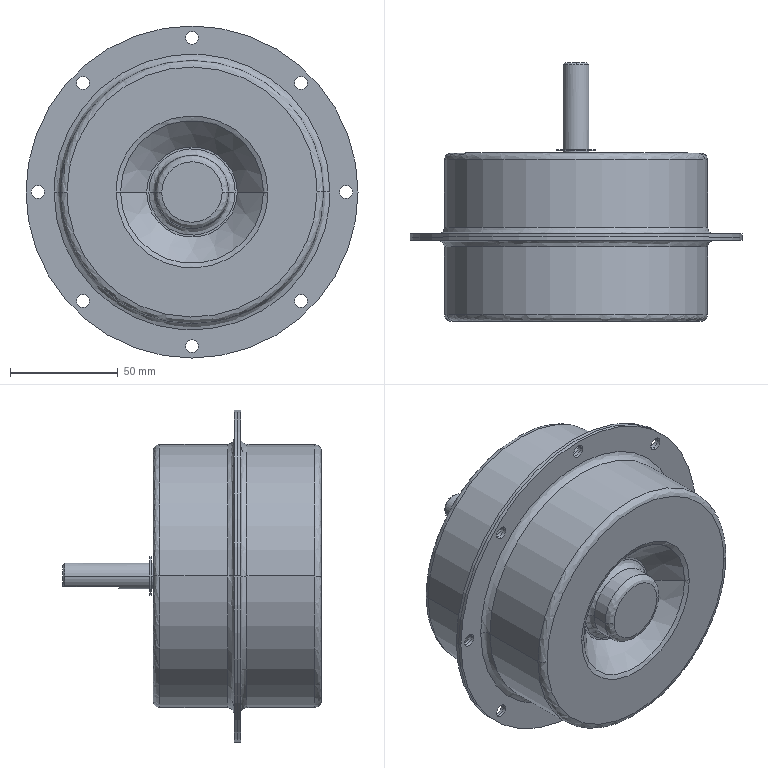Part | SolidWorks | features BaseBody 2 | 2 solids | 91 faces | box 154 x 120 x 154 mm | volume 897140 mm3 | cylinder 50 | spline 20 | plane 15 | cone 6 | commonest cylinder face diameters 6 x32 12 x4 34 x4 122 x4 154 x4 18 x2